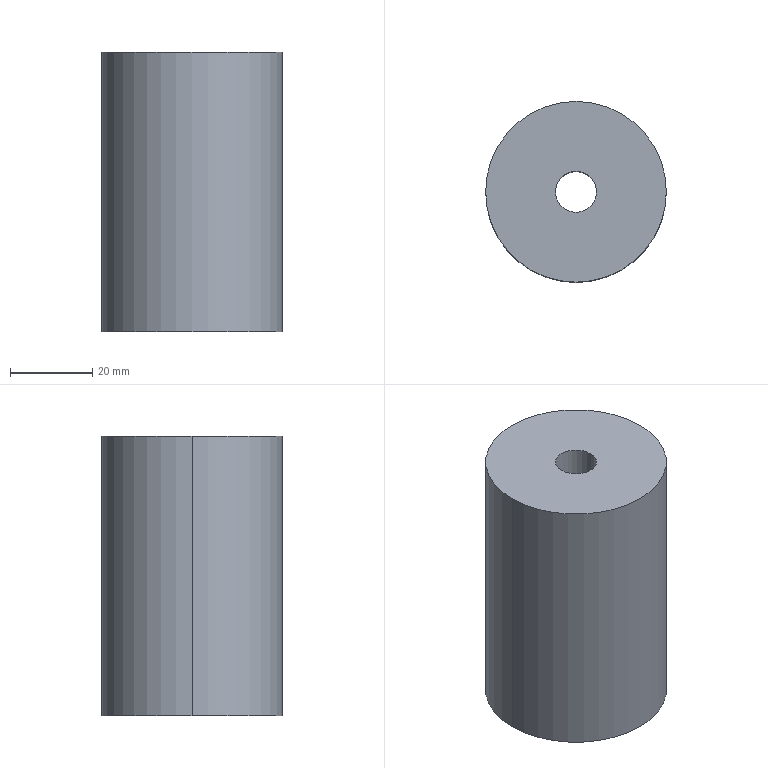Part | STEP file | 1 solid | 6 faces | box 44 x 44 x 68 mm | volume 98055 mm3 | cylinder 4 | plane 2 | commonest cylinder face diameters 10 x2 44 x2
STEP:
#1=CARTESIAN_POINT('',(0.,0.,0.));
#2=DIRECTION('',(0.,0.,1.));
#3=DIRECTION('',(1.,0.,0.));
#4=AXIS2_PLACEMENT_3D('',#1,#2,#3);
#5=CARTESIAN_POINT('',(-150.87,-201.166,-34.));
#6=VERTEX_POINT('',#5);
#7=CARTESIAN_POINT('',(-194.87,-201.166,-34.));
#8=VERTEX_POINT('',#7);
#9=CARTESIAN_POINT('',(-172.87,-201.166,-34.));
#10=DIRECTION('',(0.,0.,1.));
#11=DIRECTION('',(1.,0.,0.));
#12=AXIS2_PLACEMENT_3D('',#9,#10,#11);
#13=CIRCLE('',#12,22.);
#14=CARTESIAN_POINT('',(-172.87,-201.166,0.));
#15=DIRECTION('',(0.,0.,1.));
#16=DIRECTION('',(1.,0.,0.));
#17=AXIS2_PLACEMENT_3D('',#14,#15,#16);
#18=CYLINDRICAL_SURFACE('',#17,22.);
#19=CARTESIAN_POINT('',(0.,-34.));
#20=DIRECTION('',(1.,0.));
#21=VECTOR('',#20,1.);
#22=LINE('',#19,#21);
#23=(GEOMETRIC_REPRESENTATION_CONTEXT(2)PARAMETRIC_REPRESENTATION_CONTEXT()REPRESENTATION_CONTEXT('',''));
#24=DEFINITIONAL_REPRESENTATION('',(#22),#23);
#25=PCURVE('',#18,#24);
#26=CARTESIAN_POINT('',(-172.87,-201.166,-34.));
#27=DIRECTION('',(0.,0.,1.));
#28=DIRECTION('',(1.,0.,0.));
#29=AXIS2_PLACEMENT_3D('',#26,#27,#28);
#30=PLANE('',#29);
#31=CARTESIAN_POINT('',(0.,0.));
#32=DIRECTION('',(1.,0.));
#33=AXIS2_PLACEMENT_2D('',#31,#32);
#34=CIRCLE('',#33,22.);
#35=(GEOMETRIC_REPRESENTATION_CONTEXT(2)PARAMETRIC_REPRESENTATION_CONTEXT()REPRESENTATION_CONTEXT('',''));
#36=DEFINITIONAL_REPRESENTATION('',(#34),#35);
#37=PCURVE('',#30,#36);
#38=SURFACE_CURVE('',#13,(#25,#37),.PCURVE_S1.);
#39=EDGE_CURVE('',#6,#8,#38,.T.);
#40=ORIENTED_EDGE('',*,*,#39,.T.);
#41=CARTESIAN_POINT('',(-194.87,-201.166,34.));
#42=VERTEX_POINT('',#41);
#43=CARTESIAN_POINT('',(-194.87,-201.166,0.));
#44=DIRECTION('',(0.,0.,1.));
#45=VECTOR('',#44,1.);
#46=LINE('',#43,#45);
#47=CARTESIAN_POINT('',(3.142,0.));
#48=DIRECTION('',(0.,1.));
#49=VECTOR('',#48,1.);
#50=LINE('',#47,#49);
#51=(GEOMETRIC_REPRESENTATION_CONTEXT(2)PARAMETRIC_REPRESENTATION_CONTEXT()REPRESENTATION_CONTEXT('',''));
#52=DEFINITIONAL_REPRESENTATION('',(#50),#51);
#53=PCURVE('',#18,#52);
#54=CARTESIAN_POINT('',(-172.87,-201.166,0.));
#55=DIRECTION('',(0.,0.,1.));
#56=DIRECTION('',(1.,0.,0.));
#57=AXIS2_PLACEMENT_3D('',#54,#55,#56);
#58=CYLINDRICAL_SURFACE('',#57,22.);
#59=CARTESIAN_POINT('',(3.142,0.));
#60=DIRECTION('',(0.,1.));
#61=VECTOR('',#60,1.);
#62=LINE('',#59,#61);
#63=(GEOMETRIC_REPRESENTATION_CONTEXT(2)PARAMETRIC_REPRESENTATION_CONTEXT()REPRESENTATION_CONTEXT('',''));
#64=DEFINITIONAL_REPRESENTATION('',(#62),#63);
#65=PCURVE('',#58,#64);
#66=SURFACE_CURVE('',#46,(#53,#65),.PCURVE_S1.);
#67=EDGE_CURVE('',#8,#42,#66,.T.);
#68=ORIENTED_EDGE('',*,*,#67,.T.);
#69=CARTESIAN_POINT('',(-150.87,-201.166,34.));
#70=VERTEX_POINT('',#69);
#71=CARTESIAN_POINT('',(-172.87,-201.166,34.));
#72=DIRECTION('',(0.,0.,-1.));
#73=DIRECTION('',(1.,0.,0.));
#74=AXIS2_PLACEMENT_3D('',#71,#72,#73);
#75=CIRCLE('',#74,22.);
#76=CARTESIAN_POINT('',(6.283,34.));
#77=DIRECTION('',(-1.,0.));
#78=VECTOR('',#77,1.);
#79=LINE('',#76,#78);
#80=(GEOMETRIC_REPRESENTATION_CONTEXT(2)PARAMETRIC_REPRESENTATION_CONTEXT()REPRESENTATION_CONTEXT('',''));
#81=DEFINITIONAL_REPRESENTATION('',(#79),#80);
#82=PCURVE('',#18,#81);
#83=CARTESIAN_POINT('',(-172.87,-201.166,34.));
#84=DIRECTION('',(0.,0.,1.));
#85=DIRECTION('',(1.,0.,0.));
#86=AXIS2_PLACEMENT_3D('',#83,#84,#85);
#87=PLANE('',#86);
#88=CARTESIAN_POINT('',(22.,0.));
#89=CARTESIAN_POINT('',(22.,-38.105));
#90=CARTESIAN_POINT('',(-11.,-19.053));
#91=CARTESIAN_POINT('',(-44.,0.));
#92=CARTESIAN_POINT('',(-11.,19.053));
#93=CARTESIAN_POINT('',(22.,38.105));
#94=CARTESIAN_POINT('',(22.,0.));
#95=(BOUNDED_CURVE()B_SPLINE_CURVE(2,(#88,#89,#90,#91,#92,#93,#94),.UNSPECIFIED.,.T.,.F.)B_SPLINE_CURVE_WITH_KNOTS((1,2,2,2,2,1),(-2.094,0.,2.094,4.189,6.283,8.378),.UNSPECIFIED.)CURVE()GEOMETRIC_REPRESENTATION_ITEM()RATIONAL_B_SPLINE_CURVE((1.,0.5,1.,0.5,1.,0.5,1.))REPRESENTATION_ITEM(''));
#96=(GEOMETRIC_REPRESENTATION_CONTEXT(2)PARAMETRIC_REPRESENTATION_CONTEXT()REPRESENTATION_CONTEXT('',''));
#97=DEFINITIONAL_REPRESENTATION('',(#95),#96);
#98=PCURVE('',#87,#97);
#99=SURFACE_CURVE('',#75,(#82,#98),.PCURVE_S1.);
#100=EDGE_CURVE('',#42,#70,#99,.T.);
#101=ORIENTED_EDGE('',*,*,#100,.T.);
#102=CARTESIAN_POINT('',(-150.87,-201.166,0.));
#103=DIRECTION('',(0.,0.,1.));
#104=VECTOR('',#103,1.);
#105=LINE('',#102,#104);
#106=CARTESIAN_POINT('',(0.,0.));
#107=DIRECTION('',(0.,1.));
#108=VECTOR('',#107,1.);
#109=LINE('',#106,#108);
#110=(GEOMETRIC_REPRESENTATION_CONTEXT(2)PARAMETRIC_REPRESENTATION_CONTEXT()REPRESENTATION_CONTEXT('',''));
#111=DEFINITIONAL_REPRESENTATION('',(#109),#110);
#112=PCURVE('',#18,#111);
#113=CARTESIAN_POINT('',(6.283,0.));
#114=DIRECTION('',(0.,1.));
#115=VECTOR('',#114,1.);
#116=LINE('',#113,#115);
#117=(GEOMETRIC_REPRESENTATION_CONTEXT(2)PARAMETRIC_REPRESENTATION_CONTEXT()REPRESENTATION_CONTEXT('',''));
#118=DEFINITIONAL_REPRESENTATION('',(#116),#117);
#119=PCURVE('',#58,#118);
#120=SURFACE_CURVE('',#105,(#112,#119),.PCURVE_S1.);
#121=EDGE_CURVE('',#6,#70,#120,.T.);
#122=ORIENTED_EDGE('',*,*,#121,.F.);
#123=EDGE_LOOP('',(#40,#68,#101,#122));
#124=FACE_BOUND('',#123,.T.);
#125=ADVANCED_FACE('',(#124),#18,.T.);
#126=CARTESIAN_POINT('',(-167.87,-201.166,-34.));
#127=VERTEX_POINT('',#126);
#128=CARTESIAN_POINT('',(-167.87,-201.166,34.));
#129=VERTEX_POINT('',#128);
#130=CARTESIAN_POINT('',(-167.87,-201.166,0.));
#131=DIRECTION('',(0.,0.,1.));
#132=VECTOR('',#131,1.);
#133=LINE('',#130,#132);
#134=CARTESIAN_POINT('',(-172.87,-201.166,0.));
#135=DIRECTION('',(0.,0.,1.));
#136=DIRECTION('',(1.,0.,0.));
#137=AXIS2_PLACEMENT_3D('',#134,#135,#136);
#138=CYLINDRICAL_SURFACE('',#137,5.);
#139=CARTESIAN_POINT('',(6.283,0.));
#140=DIRECTION('',(0.,1.));
#141=VECTOR('',#140,1.);
#142=LINE('',#139,#141);
#143=(GEOMETRIC_REPRESENTATION_CONTEXT(2)PARAMETRIC_REPRESENTATION_CONTEXT()REPRESENTATION_CONTEXT('',''));
#144=DEFINITIONAL_REPRESENTATION('',(#142),#143);
#145=PCURVE('',#138,#144);
#146=CARTESIAN_POINT('',(-172.87,-201.166,0.));
#147=DIRECTION('',(0.,0.,1.));
#148=DIRECTION('',(1.,0.,0.));
#149=AXIS2_PLACEMENT_3D('',#146,#147,#148);
#150=CYLINDRICAL_SURFACE('',#149,5.);
#151=CARTESIAN_POINT('',(0.,0.));
#152=DIRECTION('',(0.,1.));
#153=VECTOR('',#152,1.);
#154=LINE('',#151,#153);
#155=(GEOMETRIC_REPRESENTATION_CONTEXT(2)PARAMETRIC_REPRESENTATION_CONTEXT()REPRESENTATION_CONTEXT('',''));
#156=DEFINITIONAL_REPRESENTATION('',(#154),#155);
#157=PCURVE('',#150,#156);
#158=SURFACE_CURVE('',#133,(#145,#157),.PCURVE_S1.);
#159=EDGE_CURVE('',#127,#129,#158,.T.);
#160=ORIENTED_EDGE('',*,*,#159,.T.);
#161=CARTESIAN_POINT('',(-177.87,-201.166,34.));
#162=VERTEX_POINT('',#161);
#163=CARTESIAN_POINT('',(-172.87,-201.166,34.));
#164=DIRECTION('',(0.,0.,-1.));
#165=DIRECTION('',(1.,0.,0.));
#166=AXIS2_PLACEMENT_3D('',#163,#164,#165);
#167=CIRCLE('',#166,5.);
#168=CARTESIAN_POINT('',(6.283,34.));
#169=DIRECTION('',(-1.,0.));
#170=VECTOR('',#169,1.);
#171=LINE('',#168,#170);
#172=(GEOMETRIC_REPRESENTATION_CONTEXT(2)PARAMETRIC_REPRESENTATION_CONTEXT()REPRESENTATION_CONTEXT('',''));
#173=DEFINITIONAL_REPRESENTATION('',(#171),#172);
#174=PCURVE('',#138,#173);
#175=CARTESIAN_POINT('',(5.,0.));
#176=CARTESIAN_POINT('',(5.,-8.66));
#177=CARTESIAN_POINT('',(-2.5,-4.33));
#178=CARTESIAN_POINT('',(-10.,0.));
#179=CARTESIAN_POINT('',(-2.5,4.33));
#180=CARTESIAN_POINT('',(5.,8.66));
#181=CARTESIAN_POINT('',(5.,0.));
#182=(BOUNDED_CURVE()B_SPLINE_CURVE(2,(#175,#176,#177,#178,#179,#180,#181),.UNSPECIFIED.,.T.,.F.)B_SPLINE_CURVE_WITH_KNOTS((1,2,2,2,2,1),(-2.094,0.,2.094,4.189,6.283,8.378),.UNSPECIFIED.)CURVE()GEOMETRIC_REPRESENTATION_ITEM()RATIONAL_B_SPLINE_CURVE((1.,0.5,1.,0.5,1.,0.5,1.))REPRESENTATION_ITEM(''));
#183=(GEOMETRIC_REPRESENTATION_CONTEXT(2)PARAMETRIC_REPRESENTATION_CONTEXT()REPRESENTATION_CONTEXT('',''));
#184=DEFINITIONAL_REPRESENTATION('',(#182),#183);
#185=PCURVE('',#87,#184);
#186=SURFACE_CURVE('',#167,(#174,#185),.PCURVE_S1.);
#187=EDGE_CURVE('',#129,#162,#186,.T.);
#188=ORIENTED_EDGE('',*,*,#187,.T.);
#189=CARTESIAN_POINT('',(-177.87,-201.166,-34.));
#190=VERTEX_POINT('',#189);
#191=CARTESIAN_POINT('',(-177.87,-201.166,0.));
#192=DIRECTION('',(0.,0.,1.));
#193=VECTOR('',#192,1.);
#194=LINE('',#191,#193);
#195=CARTESIAN_POINT('',(3.142,0.));
#196=DIRECTION('',(0.,1.));
#197=VECTOR('',#196,1.);
#198=LINE('',#195,#197);
#199=(GEOMETRIC_REPRESENTATION_CONTEXT(2)PARAMETRIC_REPRESENTATION_CONTEXT()REPRESENTATION_CONTEXT('',''));
#200=DEFINITIONAL_REPRESENTATION('',(#198),#199);
#201=PCURVE('',#138,#200);
#202=CARTESIAN_POINT('',(3.142,0.));
#203=DIRECTION('',(0.,1.));
#204=VECTOR('',#203,1.);
#205=LINE('',#202,#204);
#206=(GEOMETRIC_REPRESENTATION_CONTEXT(2)PARAMETRIC_REPRESENTATION_CONTEXT()REPRESENTATION_CONTEXT('',''));
#207=DEFINITIONAL_REPRESENTATION('',(#205),#206);
#208=PCURVE('',#150,#207);
#209=SURFACE_CURVE('',#194,(#201,#208),.PCURVE_S1.);
#210=EDGE_CURVE('',#190,#162,#209,.T.);
#211=ORIENTED_EDGE('',*,*,#210,.F.);
#212=CARTESIAN_POINT('',(-172.87,-201.166,-34.));
#213=DIRECTION('',(0.,0.,-1.));
#214=DIRECTION('',(1.,0.,0.));
#215=AXIS2_PLACEMENT_3D('',#212,#213,#214);
#216=CIRCLE('',#215,5.);
#217=CARTESIAN_POINT('',(6.283,-34.));
#218=DIRECTION('',(-1.,0.));
#219=VECTOR('',#218,1.);
#220=LINE('',#217,#219);
#221=(GEOMETRIC_REPRESENTATION_CONTEXT(2)PARAMETRIC_REPRESENTATION_CONTEXT()REPRESENTATION_CONTEXT('',''));
#222=DEFINITIONAL_REPRESENTATION('',(#220),#221);
#223=PCURVE('',#138,#222);
#224=CARTESIAN_POINT('',(5.,0.));
#225=CARTESIAN_POINT('',(5.,-8.66));
#226=CARTESIAN_POINT('',(-2.5,-4.33));
#227=CARTESIAN_POINT('',(-10.,0.));
#228=CARTESIAN_POINT('',(-2.5,4.33));
#229=CARTESIAN_POINT('',(5.,8.66));
#230=CARTESIAN_POINT('',(5.,0.));
#231=(BOUNDED_CURVE()B_SPLINE_CURVE(2,(#224,#225,#226,#227,#228,#229,#230),.UNSPECIFIED.,.T.,.F.)B_SPLINE_CURVE_WITH_KNOTS((1,2,2,2,2,1),(-2.094,0.,2.094,4.189,6.283,8.378),.UNSPECIFIED.)CURVE()GEOMETRIC_REPRESENTATION_ITEM()RATIONAL_B_SPLINE_CURVE((1.,0.5,1.,0.5,1.,0.5,1.))REPRESENTATION_ITEM(''));
#232=(GEOMETRIC_REPRESENTATION_CONTEXT(2)PARAMETRIC_REPRESENTATION_CONTEXT()REPRESENTATION_CONTEXT('',''));
#233=DEFINITIONAL_REPRESENTATION('',(#231),#232);
#234=PCURVE('',#30,#233);
#235=SURFACE_CURVE('',#216,(#223,#234),.PCURVE_S1.);
#236=EDGE_CURVE('',#127,#190,#235,.T.);
#237=ORIENTED_EDGE('',*,*,#236,.F.);
#238=EDGE_LOOP('',(#160,#188,#211,#237));
#239=FACE_BOUND('',#238,.F.);
#240=ADVANCED_FACE('',(#239),#138,.F.);
#241=ORIENTED_EDGE('',*,*,#67,.F.);
#242=CARTESIAN_POINT('',(-172.87,-201.166,-34.));
#243=DIRECTION('',(0.,0.,1.));
#244=DIRECTION('',(1.,0.,0.));
#245=AXIS2_PLACEMENT_3D('',#242,#243,#244);
#246=CIRCLE('',#245,22.);
#247=CARTESIAN_POINT('',(0.,-34.));
#248=DIRECTION('',(1.,0.));
#249=VECTOR('',#248,1.);
#250=LINE('',#247,#249);
#251=(GEOMETRIC_REPRESENTATION_CONTEXT(2)PARAMETRIC_REPRESENTATION_CONTEXT()REPRESENTATION_CONTEXT('',''));
#252=DEFINITIONAL_REPRESENTATION('',(#250),#251);
#253=PCURVE('',#58,#252);
#254=CARTESIAN_POINT('',(0.,0.));
#255=DIRECTION('',(1.,0.));
#256=AXIS2_PLACEMENT_2D('',#254,#255);
#257=CIRCLE('',#256,22.);
#258=(GEOMETRIC_REPRESENTATION_CONTEXT(2)PARAMETRIC_REPRESENTATION_CONTEXT()REPRESENTATION_CONTEXT('',''));
#259=DEFINITIONAL_REPRESENTATION('',(#257),#258);
#260=PCURVE('',#30,#259);
#261=SURFACE_CURVE('',#246,(#253,#260),.PCURVE_S1.);
#262=EDGE_CURVE('',#8,#6,#261,.T.);
#263=ORIENTED_EDGE('',*,*,#262,.T.);
#264=ORIENTED_EDGE('',*,*,#121,.T.);
#265=CARTESIAN_POINT('',(-172.87,-201.166,34.));
#266=DIRECTION('',(0.,0.,-1.));
#267=DIRECTION('',(1.,0.,0.));
#268=AXIS2_PLACEMENT_3D('',#265,#266,#267);
#269=CIRCLE('',#268,22.);
#270=CARTESIAN_POINT('',(6.283,34.));
#271=DIRECTION('',(-1.,0.));
#272=VECTOR('',#271,1.);
#273=LINE('',#270,#272);
#274=(GEOMETRIC_REPRESENTATION_CONTEXT(2)PARAMETRIC_REPRESENTATION_CONTEXT()REPRESENTATION_CONTEXT('',''));
#275=DEFINITIONAL_REPRESENTATION('',(#273),#274);
#276=PCURVE('',#58,#275);
#277=CARTESIAN_POINT('',(22.,0.));
#278=CARTESIAN_POINT('',(22.,-38.105));
#279=CARTESIAN_POINT('',(-11.,-19.053));
#280=CARTESIAN_POINT('',(-44.,0.));
#281=CARTESIAN_POINT('',(-11.,19.053));
#282=CARTESIAN_POINT('',(22.,38.105));
#283=CARTESIAN_POINT('',(22.,0.));
#284=(BOUNDED_CURVE()B_SPLINE_CURVE(2,(#277,#278,#279,#280,#281,#282,#283),.UNSPECIFIED.,.T.,.F.)B_SPLINE_CURVE_WITH_KNOTS((1,2,2,2,2,1),(-2.094,0.,2.094,4.189,6.283,8.378),.UNSPECIFIED.)CURVE()GEOMETRIC_REPRESENTATION_ITEM()RATIONAL_B_SPLINE_CURVE((1.,0.5,1.,0.5,1.,0.5,1.))REPRESENTATION_ITEM(''));
#285=(GEOMETRIC_REPRESENTATION_CONTEXT(2)PARAMETRIC_REPRESENTATION_CONTEXT()REPRESENTATION_CONTEXT('',''));
#286=DEFINITIONAL_REPRESENTATION('',(#284),#285);
#287=PCURVE('',#87,#286);
#288=SURFACE_CURVE('',#269,(#276,#287),.PCURVE_S1.);
#289=EDGE_CURVE('',#70,#42,#288,.T.);
#290=ORIENTED_EDGE('',*,*,#289,.T.);
#291=EDGE_LOOP('',(#241,#263,#264,#290));
#292=FACE_BOUND('',#291,.T.);
#293=ADVANCED_FACE('',(#292),#58,.T.);
#294=ORIENTED_EDGE('',*,*,#289,.F.);
#295=ORIENTED_EDGE('',*,*,#100,.F.);
#296=EDGE_LOOP('',(#294,#295));
#297=FACE_BOUND('',#296,.T.);
#298=ORIENTED_EDGE('',*,*,#187,.T.);
#299=CARTESIAN_POINT('',(-172.87,-201.166,34.));
#300=DIRECTION('',(0.,0.,-1.));
#301=DIRECTION('',(1.,0.,0.));
#302=AXIS2_PLACEMENT_3D('',#299,#300,#301);
#303=CIRCLE('',#302,5.);
#304=CARTESIAN_POINT('',(5.,0.));
#305=CARTESIAN_POINT('',(5.,-8.66));
#306=CARTESIAN_POINT('',(-2.5,-4.33));
#307=CARTESIAN_POINT('',(-10.,0.));
#308=CARTESIAN_POINT('',(-2.5,4.33));
#309=CARTESIAN_POINT('',(5.,8.66));
#310=CARTESIAN_POINT('',(5.,0.));
#311=(BOUNDED_CURVE()B_SPLINE_CURVE(2,(#304,#305,#306,#307,#308,#309,#310),.UNSPECIFIED.,.T.,.F.)B_SPLINE_CURVE_WITH_KNOTS((1,2,2,2,2,1),(-2.094,0.,2.094,4.189,6.283,8.378),.UNSPECIFIED.)CURVE()GEOMETRIC_REPRESENTATION_ITEM()RATIONAL_B_SPLINE_CURVE((1.,0.5,1.,0.5,1.,0.5,1.))REPRESENTATION_ITEM(''));
#312=(GEOMETRIC_REPRESENTATION_CONTEXT(2)PARAMETRIC_REPRESENTATION_CONTEXT()REPRESENTATION_CONTEXT('',''));
#313=DEFINITIONAL_REPRESENTATION('',(#311),#312);
#314=PCURVE('',#87,#313);
#315=CARTESIAN_POINT('',(6.283,34.));
#316=DIRECTION('',(-1.,0.));
#317=VECTOR('',#316,1.);
#318=LINE('',#315,#317);
#319=(GEOMETRIC_REPRESENTATION_CONTEXT(2)PARAMETRIC_REPRESENTATION_CONTEXT()REPRESENTATION_CONTEXT('',''));
#320=DEFINITIONAL_REPRESENTATION('',(#318),#319);
#321=PCURVE('',#150,#320);
#322=SURFACE_CURVE('',#303,(#314,#321),.PCURVE_S1.);
#323=EDGE_CURVE('',#162,#129,#322,.T.);
#324=ORIENTED_EDGE('',*,*,#323,.T.);
#325=EDGE_LOOP('',(#298,#324));
#326=FACE_BOUND('',#325,.T.);
#327=ADVANCED_FACE('',(#297,#326),#87,.T.);
#328=ORIENTED_EDGE('',*,*,#39,.F.);
#329=ORIENTED_EDGE('',*,*,#262,.F.);
#330=EDGE_LOOP('',(#328,#329));
#331=FACE_BOUND('',#330,.T.);
#332=ORIENTED_EDGE('',*,*,#236,.F.);
#333=CARTESIAN_POINT('',(-172.87,-201.166,-34.));
#334=DIRECTION('',(0.,0.,-1.));
#335=DIRECTION('',(1.,0.,0.));
#336=AXIS2_PLACEMENT_3D('',#333,#334,#335);
#337=CIRCLE('',#336,5.);
#338=CARTESIAN_POINT('',(5.,0.));
#339=CARTESIAN_POINT('',(5.,-8.66));
#340=CARTESIAN_POINT('',(-2.5,-4.33));
#341=CARTESIAN_POINT('',(-10.,0.));
#342=CARTESIAN_POINT('',(-2.5,4.33));
#343=CARTESIAN_POINT('',(5.,8.66));
#344=CARTESIAN_POINT('',(5.,0.));
#345=(BOUNDED_CURVE()B_SPLINE_CURVE(2,(#338,#339,#340,#341,#342,#343,#344),.UNSPECIFIED.,.T.,.F.)B_SPLINE_CURVE_WITH_KNOTS((1,2,2,2,2,1),(-2.094,0.,2.094,4.189,6.283,8.378),.UNSPECIFIED.)CURVE()GEOMETRIC_REPRESENTATION_ITEM()RATIONAL_B_SPLINE_CURVE((1.,0.5,1.,0.5,1.,0.5,1.))REPRESENTATION_ITEM(''));
#346=(GEOMETRIC_REPRESENTATION_CONTEXT(2)PARAMETRIC_REPRESENTATION_CONTEXT()REPRESENTATION_CONTEXT('',''));
#347=DEFINITIONAL_REPRESENTATION('',(#345),#346);
#348=PCURVE('',#30,#347);
#349=CARTESIAN_POINT('',(6.283,-34.));
#350=DIRECTION('',(-1.,0.));
#351=VECTOR('',#350,1.);
#352=LINE('',#349,#351);
#353=(GEOMETRIC_REPRESENTATION_CONTEXT(2)PARAMETRIC_REPRESENTATION_CONTEXT()REPRESENTATION_CONTEXT('',''));
#354=DEFINITIONAL_REPRESENTATION('',(#352),#353);
#355=PCURVE('',#150,#354);
#356=SURFACE_CURVE('',#337,(#348,#355),.PCURVE_S1.);
#357=EDGE_CURVE('',#190,#127,#356,.T.);
#358=ORIENTED_EDGE('',*,*,#357,.F.);
#359=EDGE_LOOP('',(#332,#358));
#360=FACE_BOUND('',#359,.T.);
#361=ADVANCED_FACE('',(#331,#360),#30,.F.);
#362=ORIENTED_EDGE('',*,*,#323,.T.);
#363=ORIENTED_EDGE('',*,*,#159,.F.);
#364=ORIENTED_EDGE('',*,*,#357,.F.);
#365=ORIENTED_EDGE('',*,*,#210,.T.);
#366=EDGE_LOOP('',(#362,#363,#364,#365));
#367=FACE_BOUND('',#366,.F.);
#368=ADVANCED_FACE('',(#367),#150,.F.);
#369=CLOSED_SHELL('',(#125,#240,#293,#327,#361,#368));
#370=MANIFOLD_SOLID_BREP('',#369);
#371=(LENGTH_UNIT()NAMED_UNIT(*)SI_UNIT(.MILLI.,.METRE.));
#372=UNCERTAINTY_MEASURE_WITH_UNIT(LENGTH_MEASURE(0.0000001),#371,'','');
#373=(NAMED_UNIT(*)PLANE_ANGLE_UNIT()SI_UNIT($,.RADIAN.));
#374=(NAMED_UNIT(*)SI_UNIT($,.STERADIAN.)SOLID_ANGLE_UNIT());
#375=(GEOMETRIC_REPRESENTATION_CONTEXT(3)GLOBAL_UNCERTAINTY_ASSIGNED_CONTEXT((#372))GLOBAL_UNIT_ASSIGNED_CONTEXT((#371,#373,#374))REPRESENTATION_CONTEXT('',''));
#376=ADVANCED_BREP_SHAPE_REPRESENTATION('',(#4,#370),#375);